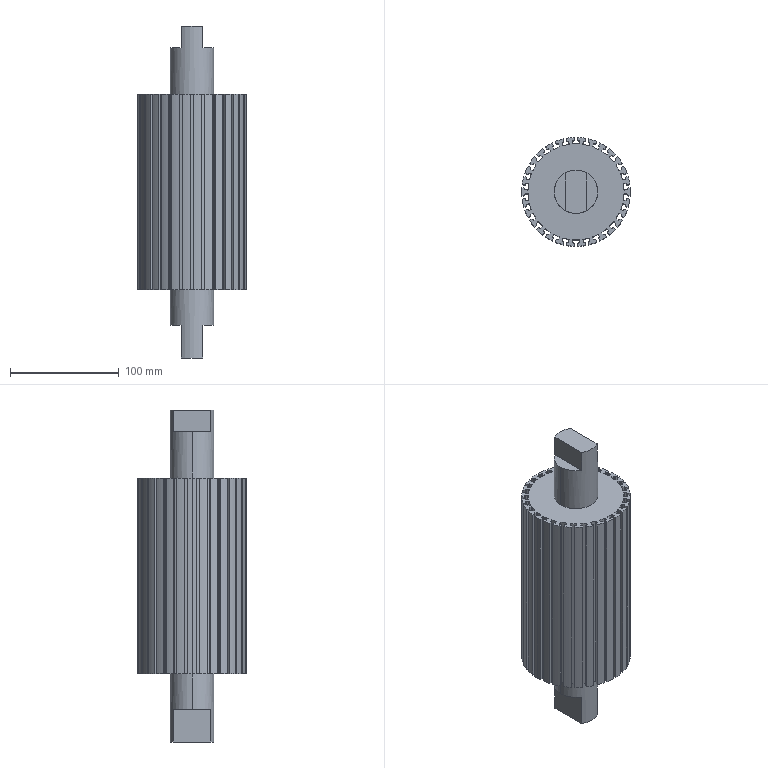Part | SolidWorks | 1 solid | 479 faces | box 100 x 99.955 x 305 mm | volume 1401130 mm3 | cylinder 257 | plane 222 | commonest cylinder face diameters 1 x222 100 x31 40 x4